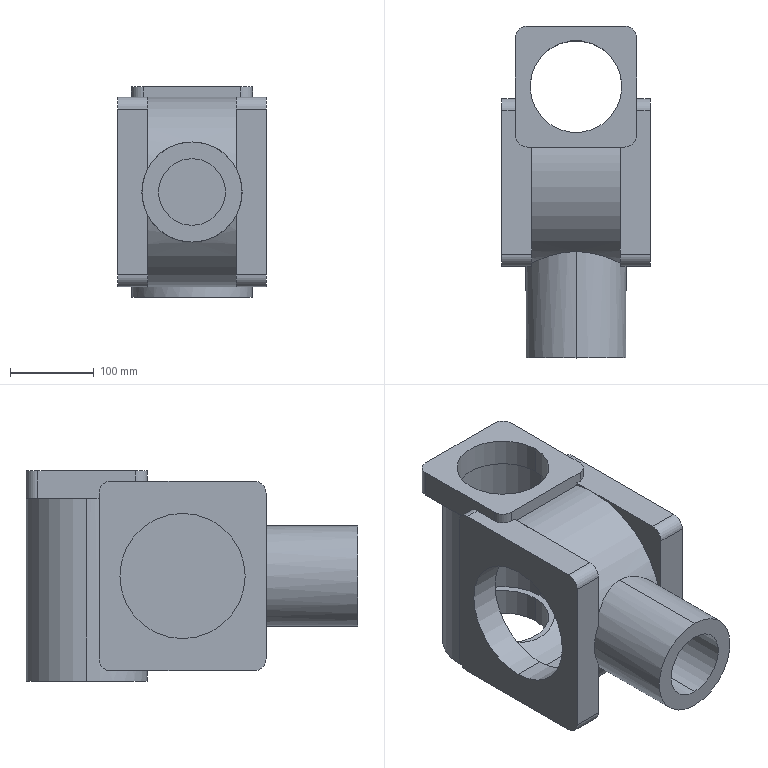Part | SolidWorks | features ICE 12, Extrusion 1, Fillet 1 | 1 solid | 69 faces | box 178 x 397.308 x 252 mm | volume 4609278 mm3 | plane 35 | cylinder 34 | commonest cylinder face diameters 28.4 x12 110 x4 150 x4 198 x3 227 x3 80 x2